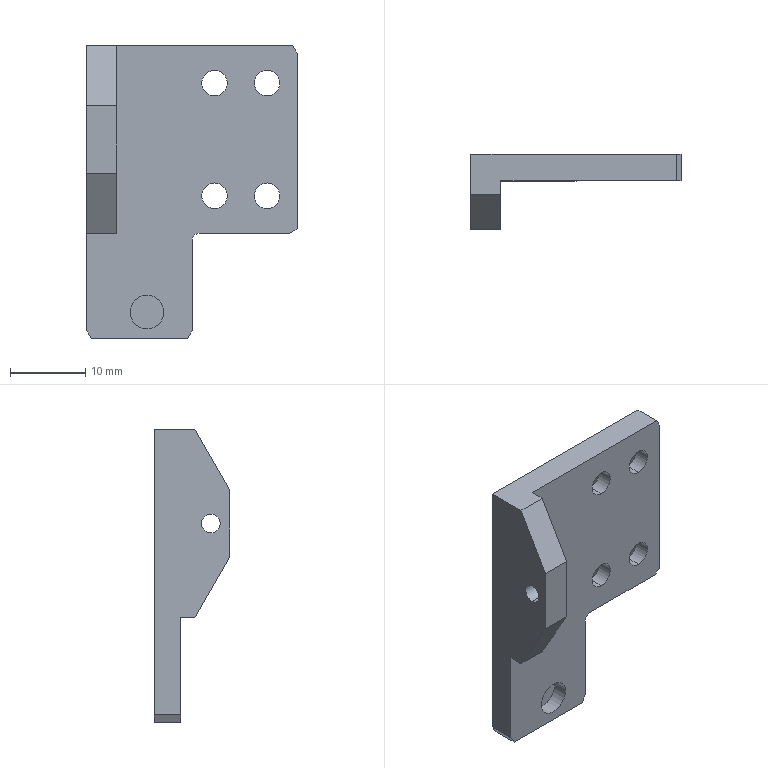Part | NX | features BREP 1 | 1 solid | 39 faces | box 28 x 10 x 39 mm | volume 3399 mm3 | plane 18 | cylinder 13 | cone 8 | commonest cylinder face diameters 3.4 x8 2.5 x2 4.5 x2 2 x1
STEP:
#1=CARTESIAN_POINT('',(15.,10.,-12.5));
#2=VERTEX_POINT('',#1);
#3=CARTESIAN_POINT('',(14.,10.,-13.5));
#4=VERTEX_POINT('',#3);
#5=CARTESIAN_POINT('',(15.,10.,-13.5));
#6=DIRECTION('',(0.,-1.,0.));
#7=DIRECTION('',(0.,0.,-1.));
#8=AXIS2_PLACEMENT_3D('',#5,#6,#7);
#9=CIRCLE('',#8,1.);
#10=EDGE_CURVE('',#2,#4,#9,.T.);
#11=ORIENTED_EDGE('',*,*,#10,.F.);
#12=CARTESIAN_POINT('',(15.,6.5,-12.5));
#13=VERTEX_POINT('',#12);
#14=CARTESIAN_POINT('',(15.,0.,-12.5));
#15=DIRECTION('',(0.,1.,0.));
#16=VECTOR('',#15,1000.);
#17=LINE('',#14,#16);
#18=EDGE_CURVE('',#13,#2,#17,.T.);
#19=ORIENTED_EDGE('',*,*,#18,.F.);
#20=CARTESIAN_POINT('',(14.,6.5,-13.5));
#21=VERTEX_POINT('',#20);
#22=CARTESIAN_POINT('',(15.,6.5,-13.5));
#23=DIRECTION('',(0.,1.,0.));
#24=DIRECTION('',(-1.,0.,0.));
#25=AXIS2_PLACEMENT_3D('',#22,#23,#24);
#26=CIRCLE('',#25,1.);
#27=EDGE_CURVE('',#21,#13,#26,.T.);
#28=ORIENTED_EDGE('',*,*,#27,.F.);
#29=CARTESIAN_POINT('',(14.,10.,-13.5));
#30=DIRECTION('',(0.,-1.,0.));
#31=VECTOR('',#30,1000.);
#32=LINE('',#29,#31);
#33=EDGE_CURVE('',#4,#21,#32,.T.);
#34=ORIENTED_EDGE('',*,*,#33,.F.);
#35=EDGE_LOOP('',(#11,#19,#28,#34));
#36=FACE_BOUND('',#35,.T.);
#37=CARTESIAN_POINT('',(15.,10.,-13.5));
#38=DIRECTION('',(0.,-1.,0.));
#39=DIRECTION('',(1.,0.,0.));
#40=AXIS2_PLACEMENT_3D('',#37,#38,#39);
#41=CYLINDRICAL_SURFACE('',#40,1.);
#42=ADVANCED_FACE('',(#36),#41,.F.);
#43=CARTESIAN_POINT('',(14.,10.,-25.5));
#44=VERTEX_POINT('',#43);
#45=CARTESIAN_POINT('',(13.423,10.,-26.5));
#46=VERTEX_POINT('',#45);
#47=CARTESIAN_POINT('',(13.423,10.,-26.5));
#48=DIRECTION('',(-0.5,0.,-0.866));
#49=VECTOR('',#48,1000.);
#50=LINE('',#47,#49);
#51=EDGE_CURVE('',#44,#46,#50,.T.);
#52=ORIENTED_EDGE('',*,*,#51,.F.);
#53=CARTESIAN_POINT('',(14.,6.5,-25.5));
#54=VERTEX_POINT('',#53);
#55=CARTESIAN_POINT('',(14.,10.,-25.5));
#56=DIRECTION('',(0.,1.,0.));
#57=VECTOR('',#56,1000.);
#58=LINE('',#55,#57);
#59=EDGE_CURVE('',#54,#44,#58,.T.);
#60=ORIENTED_EDGE('',*,*,#59,.F.);
#61=CARTESIAN_POINT('',(13.423,6.5,-26.5));
#62=VERTEX_POINT('',#61);
#63=CARTESIAN_POINT('',(13.423,6.5,-26.5));
#64=DIRECTION('',(0.5,0.,0.866));
#65=VECTOR('',#64,1000.);
#66=LINE('',#63,#65);
#67=EDGE_CURVE('',#62,#54,#66,.T.);
#68=ORIENTED_EDGE('',*,*,#67,.F.);
#69=CARTESIAN_POINT('',(13.423,0.,-26.5));
#70=DIRECTION('',(0.,-1.,0.));
#71=VECTOR('',#70,1000.);
#72=LINE('',#69,#71);
#73=EDGE_CURVE('',#46,#62,#72,.T.);
#74=ORIENTED_EDGE('',*,*,#73,.F.);
#75=EDGE_LOOP('',(#52,#60,#68,#74));
#76=FACE_BOUND('',#75,.T.);
#77=CARTESIAN_POINT('',(13.423,0.,-26.5));
#78=DIRECTION('',(-0.866,0.,0.5));
#79=DIRECTION('',(0.,-1.,0.));
#80=AXIS2_PLACEMENT_3D('',#77,#78,#79);
#81=PLANE('',#80);
#82=ADVANCED_FACE('',(#76),#81,.F.);
#83=CARTESIAN_POINT('',(0.,6.5,-25.5));
#84=VERTEX_POINT('',#83);
#85=CARTESIAN_POINT('',(0.5774,6.5,-26.5));
#86=VERTEX_POINT('',#85);
#87=CARTESIAN_POINT('',(0.5774,6.5,-26.5));
#88=DIRECTION('',(0.5,0.,-0.866));
#89=VECTOR('',#88,1000.);
#90=LINE('',#87,#89);
#91=EDGE_CURVE('',#84,#86,#90,.T.);
#92=ORIENTED_EDGE('',*,*,#91,.F.);
#93=CARTESIAN_POINT('',(0.,10.,-25.5));
#94=VERTEX_POINT('',#93);
#95=CARTESIAN_POINT('',(0.,0.,-25.5));
#96=DIRECTION('',(0.,-1.,0.));
#97=VECTOR('',#96,1000.);
#98=LINE('',#95,#97);
#99=EDGE_CURVE('',#94,#84,#98,.T.);
#100=ORIENTED_EDGE('',*,*,#99,.F.);
#101=CARTESIAN_POINT('',(0.5774,10.,-26.5));
#102=VERTEX_POINT('',#101);
#103=CARTESIAN_POINT('',(0.5774,10.,-26.5));
#104=DIRECTION('',(-0.5,0.,0.866));
#105=VECTOR('',#104,1000.);
#106=LINE('',#103,#105);
#107=EDGE_CURVE('',#102,#94,#106,.T.);
#108=ORIENTED_EDGE('',*,*,#107,.F.);
#109=CARTESIAN_POINT('',(0.5774,0.,-26.5));
#110=DIRECTION('',(0.,1.,0.));
#111=VECTOR('',#110,1000.);
#112=LINE('',#109,#111);
#113=EDGE_CURVE('',#86,#102,#112,.T.);
#114=ORIENTED_EDGE('',*,*,#113,.F.);
#115=EDGE_LOOP('',(#92,#100,#108,#114));
#116=FACE_BOUND('',#115,.T.);
#117=CARTESIAN_POINT('',(0.5774,0.,-26.5));
#118=DIRECTION('',(0.866,0.,0.5));
#119=DIRECTION('',(0.,1.,0.));
#120=AXIS2_PLACEMENT_3D('',#117,#118,#119);
#121=PLANE('',#120);
#122=ADVANCED_FACE('',(#116),#121,.F.);
#123=CARTESIAN_POINT('',(27.,6.5,-12.5));
#124=VERTEX_POINT('',#123);
#125=CARTESIAN_POINT('',(28.,6.5,-11.923));
#126=VERTEX_POINT('',#125);
#127=CARTESIAN_POINT('',(28.,6.5,-11.923));
#128=DIRECTION('',(0.866,0.,0.5));
#129=VECTOR('',#128,1000.);
#130=LINE('',#127,#129);
#131=EDGE_CURVE('',#124,#126,#130,.T.);
#132=ORIENTED_EDGE('',*,*,#131,.F.);
#133=CARTESIAN_POINT('',(27.,10.,-12.5));
#134=VERTEX_POINT('',#133);
#135=CARTESIAN_POINT('',(27.,6.5,-12.5));
#136=DIRECTION('',(0.,-1.,0.));
#137=VECTOR('',#136,1000.);
#138=LINE('',#135,#137);
#139=EDGE_CURVE('',#134,#124,#138,.T.);
#140=ORIENTED_EDGE('',*,*,#139,.F.);
#141=CARTESIAN_POINT('',(28.,10.,-11.923));
#142=VERTEX_POINT('',#141);
#143=CARTESIAN_POINT('',(28.,10.,-11.923));
#144=DIRECTION('',(-0.866,0.,-0.5));
#145=VECTOR('',#144,1000.);
#146=LINE('',#143,#145);
#147=EDGE_CURVE('',#142,#134,#146,.T.);
#148=ORIENTED_EDGE('',*,*,#147,.F.);
#149=CARTESIAN_POINT('',(28.,10.,-11.923));
#150=DIRECTION('',(0.,1.,0.));
#151=VECTOR('',#150,1000.);
#152=LINE('',#149,#151);
#153=EDGE_CURVE('',#126,#142,#152,.T.);
#154=ORIENTED_EDGE('',*,*,#153,.F.);
#155=EDGE_LOOP('',(#132,#140,#148,#154));
#156=FACE_BOUND('',#155,.T.);
#157=CARTESIAN_POINT('',(28.,10.,-11.923));
#158=DIRECTION('',(0.5,0.,-0.866));
#159=DIRECTION('',(0.,-1.,0.));
#160=AXIS2_PLACEMENT_3D('',#157,#158,#159);
#161=PLANE('',#160);
#162=ADVANCED_FACE('',(#156),#161,.T.);
#163=CARTESIAN_POINT('',(28.,6.5,11.5));
#164=VERTEX_POINT('',#163);
#165=CARTESIAN_POINT('',(27.423,6.5,12.5));
#166=VERTEX_POINT('',#165);
#167=CARTESIAN_POINT('',(27.423,6.5,12.5));
#168=DIRECTION('',(-0.5,0.,0.866));
#169=VECTOR('',#168,1000.);
#170=LINE('',#167,#169);
#171=EDGE_CURVE('',#164,#166,#170,.T.);
#172=ORIENTED_EDGE('',*,*,#171,.F.);
#173=CARTESIAN_POINT('',(28.,10.,11.5));
#174=VERTEX_POINT('',#173);
#175=CARTESIAN_POINT('',(28.,10.,11.5));
#176=DIRECTION('',(0.,-1.,0.));
#177=VECTOR('',#176,1000.);
#178=LINE('',#175,#177);
#179=EDGE_CURVE('',#174,#164,#178,.T.);
#180=ORIENTED_EDGE('',*,*,#179,.F.);
#181=CARTESIAN_POINT('',(27.423,10.,12.5));
#182=VERTEX_POINT('',#181);
#183=CARTESIAN_POINT('',(27.423,10.,12.5));
#184=DIRECTION('',(0.5,0.,-0.866));
#185=VECTOR('',#184,1000.);
#186=LINE('',#183,#185);
#187=EDGE_CURVE('',#182,#174,#186,.T.);
#188=ORIENTED_EDGE('',*,*,#187,.F.);
#189=CARTESIAN_POINT('',(27.423,0.,12.5));
#190=DIRECTION('',(0.,1.,0.));
#191=VECTOR('',#190,1000.);
#192=LINE('',#189,#191);
#193=EDGE_CURVE('',#166,#182,#192,.T.);
#194=ORIENTED_EDGE('',*,*,#193,.F.);
#195=EDGE_LOOP('',(#172,#180,#188,#194));
#196=FACE_BOUND('',#195,.T.);
#197=CARTESIAN_POINT('',(27.423,0.,12.5));
#198=DIRECTION('',(-0.866,0.,-0.5));
#199=DIRECTION('',(0.,1.,0.));
#200=AXIS2_PLACEMENT_3D('',#197,#198,#199);
#201=PLANE('',#200);
#202=ADVANCED_FACE('',(#196),#201,.F.);
#203=CARTESIAN_POINT('',(10.25,8.5,-23.));
#204=VERTEX_POINT('',#203);
#205=CARTESIAN_POINT('',(5.75,8.5,-23.));
#206=VERTEX_POINT('',#205);
#207=CARTESIAN_POINT('',(8.,8.5,-23.));
#208=DIRECTION('',(0.,-1.,0.));
#209=DIRECTION('',(1.,0.,0.));
#210=AXIS2_PLACEMENT_3D('',#207,#208,#209);
#211=CIRCLE('',#210,2.25);
#212=EDGE_CURVE('',#204,#206,#211,.T.);
#213=ORIENTED_EDGE('',*,*,#212,.T.);
#214=CARTESIAN_POINT('',(8.,8.5,-23.));
#215=DIRECTION('',(0.,-1.,0.));
#216=DIRECTION('',(1.,0.,0.));
#217=AXIS2_PLACEMENT_3D('',#214,#215,#216);
#218=CIRCLE('',#217,2.25);
#219=EDGE_CURVE('',#206,#204,#218,.T.);
#220=ORIENTED_EDGE('',*,*,#219,.T.);
#221=EDGE_LOOP('',(#213,#220));
#222=FACE_BOUND('',#221,.T.);
#223=CARTESIAN_POINT('',(8.,8.5,-23.));
#224=DIRECTION('',(0.,-1.,0.));
#225=DIRECTION('',(1.,0.,0.));
#226=AXIS2_PLACEMENT_3D('',#223,#224,#225);
#227=PLANE('',#226);
#228=ADVANCED_FACE('',(#222),#227,.T.);
#229=CARTESIAN_POINT('',(5.75,6.5,-23.));
#230=VERTEX_POINT('',#229);
#231=CARTESIAN_POINT('',(5.75,8.5,-23.));
#232=DIRECTION('',(0.,-1.,0.));
#233=VECTOR('',#232,1000.);
#234=LINE('',#231,#233);
#235=EDGE_CURVE('',#230,#206,#234,.F.);
#236=ORIENTED_EDGE('',*,*,#235,.T.);
#237=ORIENTED_EDGE('',*,*,#212,.F.);
#238=CARTESIAN_POINT('',(10.25,6.5,-23.));
#239=VERTEX_POINT('',#238);
#240=CARTESIAN_POINT('',(10.25,8.5,-23.));
#241=DIRECTION('',(0.,-1.,0.));
#242=VECTOR('',#241,1000.);
#243=LINE('',#240,#242);
#244=EDGE_CURVE('',#239,#204,#243,.F.);
#245=ORIENTED_EDGE('',*,*,#244,.F.);
#246=CARTESIAN_POINT('',(8.,6.5,-23.));
#247=DIRECTION('',(0.,-1.,0.));
#248=DIRECTION('',(1.,0.,0.));
#249=AXIS2_PLACEMENT_3D('',#246,#247,#248);
#250=CIRCLE('',#249,2.25);
#251=EDGE_CURVE('',#239,#230,#250,.T.);
#252=ORIENTED_EDGE('',*,*,#251,.T.);
#253=EDGE_LOOP('',(#236,#237,#245,#252));
#254=FACE_BOUND('',#253,.T.);
#255=CARTESIAN_POINT('',(8.,8.5,-23.));
#256=DIRECTION('',(0.,-1.,0.));
#257=DIRECTION('',(1.,0.,0.));
#258=AXIS2_PLACEMENT_3D('',#255,#256,#257);
#259=CYLINDRICAL_SURFACE('',#258,2.25);
#260=ADVANCED_FACE('',(#254),#259,.F.);
#261=CARTESIAN_POINT('',(0.,6.5,-26.5));
#262=DIRECTION('',(-1.,0.,0.));
#263=VECTOR('',#262,1000.);
#264=LINE('',#261,#263);
#265=EDGE_CURVE('',#62,#86,#264,.T.);
#266=ORIENTED_EDGE('',*,*,#265,.T.);
#267=ORIENTED_EDGE('',*,*,#113,.T.);
#268=CARTESIAN_POINT('',(0.,10.,-26.5));
#269=DIRECTION('',(1.,0.,0.));
#270=VECTOR('',#269,1000.);
#271=LINE('',#268,#270);
#272=EDGE_CURVE('',#102,#46,#271,.T.);
#273=ORIENTED_EDGE('',*,*,#272,.T.);
#274=ORIENTED_EDGE('',*,*,#73,.T.);
#275=EDGE_LOOP('',(#266,#267,#273,#274));
#276=FACE_BOUND('',#275,.T.);
#277=CARTESIAN_POINT('',(0.,0.,-26.5));
#278=DIRECTION('',(0.,0.,1.));
#279=DIRECTION('',(1.,0.,0.));
#280=AXIS2_PLACEMENT_3D('',#277,#278,#279);
#281=PLANE('',#280);
#282=ADVANCED_FACE('',(#276),#281,.F.);
#283=CARTESIAN_POINT('',(14.,10.,-26.5));
#284=DIRECTION('',(0.,0.,1.));
#285=VECTOR('',#284,1000.);
#286=LINE('',#283,#285);
#287=EDGE_CURVE('',#44,#4,#286,.T.);
#288=ORIENTED_EDGE('',*,*,#287,.T.);
#289=ORIENTED_EDGE('',*,*,#33,.T.);
#290=CARTESIAN_POINT('',(14.,6.5,-26.5));
#291=DIRECTION('',(0.,0.,1.));
#292=VECTOR('',#291,1000.);
#293=LINE('',#290,#292);
#294=EDGE_CURVE('',#54,#21,#293,.T.);
#295=ORIENTED_EDGE('',*,*,#294,.F.);
#296=ORIENTED_EDGE('',*,*,#59,.T.);
#297=EDGE_LOOP('',(#288,#289,#295,#296));
#298=FACE_BOUND('',#297,.T.);
#299=CARTESIAN_POINT('',(14.,10.,-26.5));
#300=DIRECTION('',(-1.,0.,0.));
#301=DIRECTION('',(0.,-1.,0.));
#302=AXIS2_PLACEMENT_3D('',#299,#300,#301);
#303=PLANE('',#302);
#304=ADVANCED_FACE('',(#298),#303,.F.);
#305=CARTESIAN_POINT('',(0.,0.,4.5));
#306=VERTEX_POINT('',#305);
#307=CARTESIAN_POINT('',(0.,4.619,12.5));
#308=VERTEX_POINT('',#307);
#309=CARTESIAN_POINT('',(0.,4.619,12.5));
#310=DIRECTION('',(0.,0.5,0.866));
#311=VECTOR('',#310,1000.);
#312=LINE('',#309,#311);
#313=EDGE_CURVE('',#306,#308,#312,.T.);
#314=ORIENTED_EDGE('',*,*,#313,.F.);
#315=CARTESIAN_POINT('',(4.,0.,4.5));
#316=VERTEX_POINT('',#315);
#317=CARTESIAN_POINT('',(4.,0.,4.5));
#318=DIRECTION('',(-1.,0.,0.));
#319=VECTOR('',#318,1000.);
#320=LINE('',#317,#319);
#321=EDGE_CURVE('',#316,#306,#320,.T.);
#322=ORIENTED_EDGE('',*,*,#321,.F.);
#323=CARTESIAN_POINT('',(4.,4.619,12.5));
#324=VERTEX_POINT('',#323);
#325=CARTESIAN_POINT('',(4.,4.619,12.5));
#326=DIRECTION('',(0.,-0.5,-0.866));
#327=VECTOR('',#326,1000.);
#328=LINE('',#325,#327);
#329=EDGE_CURVE('',#324,#316,#328,.T.);
#330=ORIENTED_EDGE('',*,*,#329,.F.);
#331=CARTESIAN_POINT('',(0.,4.619,12.5));
#332=DIRECTION('',(1.,0.,0.));
#333=VECTOR('',#332,1000.);
#334=LINE('',#331,#333);
#335=EDGE_CURVE('',#308,#324,#334,.T.);
#336=ORIENTED_EDGE('',*,*,#335,.F.);
#337=EDGE_LOOP('',(#314,#322,#330,#336));
#338=FACE_BOUND('',#337,.T.);
#339=CARTESIAN_POINT('',(0.,4.619,12.5));
#340=DIRECTION('',(0.,0.866,-0.5));
#341=DIRECTION('',(1.,0.,0.));
#342=AXIS2_PLACEMENT_3D('',#339,#340,#341);
#343=PLANE('',#342);
#344=ADVANCED_FACE('',(#338),#343,.F.);
#345=CARTESIAN_POINT('',(0.,4.619,-12.5));
#346=VERTEX_POINT('',#345);
#347=CARTESIAN_POINT('',(0.,0.,-4.5));
#348=VERTEX_POINT('',#347);
#349=CARTESIAN_POINT('',(0.,0.,-4.5));
#350=DIRECTION('',(0.,-0.5,0.866));
#351=VECTOR('',#350,1000.);
#352=LINE('',#349,#351);
#353=EDGE_CURVE('',#346,#348,#352,.T.);
#354=ORIENTED_EDGE('',*,*,#353,.F.);
#355=CARTESIAN_POINT('',(4.,4.619,-12.5));
#356=VERTEX_POINT('',#355);
#357=CARTESIAN_POINT('',(0.,4.619,-12.5));
#358=DIRECTION('',(-1.,0.,0.));
#359=VECTOR('',#358,1000.);
#360=LINE('',#357,#359);
#361=EDGE_CURVE('',#356,#346,#360,.T.);
#362=ORIENTED_EDGE('',*,*,#361,.F.);
#363=CARTESIAN_POINT('',(4.,0.,-4.5));
#364=VERTEX_POINT('',#363);
#365=CARTESIAN_POINT('',(4.,0.,-4.5));
#366=DIRECTION('',(0.,0.5,-0.866));
#367=VECTOR('',#366,1000.);
#368=LINE('',#365,#367);
#369=EDGE_CURVE('',#364,#356,#368,.T.);
#370=ORIENTED_EDGE('',*,*,#369,.F.);
#371=CARTESIAN_POINT('',(4.,0.,-4.5));
#372=DIRECTION('',(1.,0.,0.));
#373=VECTOR('',#372,1000.);
#374=LINE('',#371,#373);
#375=EDGE_CURVE('',#348,#364,#374,.T.);
#376=ORIENTED_EDGE('',*,*,#375,.F.);
#377=EDGE_LOOP('',(#354,#362,#370,#376));
#378=FACE_BOUND('',#377,.T.);
#379=CARTESIAN_POINT('',(4.,0.,-4.5));
#380=DIRECTION('',(0.,-0.866,-0.5));
#381=DIRECTION('',(-1.,0.,0.));
#382=AXIS2_PLACEMENT_3D('',#379,#380,#381);
#383=PLANE('',#382);
#384=ADVANCED_FACE('',(#378),#383,.T.);
#385=CARTESIAN_POINT('',(17.,10.,4.35));
#386=VERTEX_POINT('',#385);
#387=CARTESIAN_POINT('',(17.,8.55,5.8));
#388=VERTEX_POINT('',#387);
#389=CARTESIAN_POINT('',(17.,10.,4.35));
#390=DIRECTION('',(0.,0.7071,-0.7071));
#391=VECTOR('',#390,1000.);
#392=LINE('',#389,#391);
#393=EDGE_CURVE('',#386,#388,#392,.F.);
#394=ORIENTED_EDGE('',*,*,#393,.T.);
#395=CARTESIAN_POINT('',(17.,8.55,9.2));
#396=VERTEX_POINT('',#395);
#397=CARTESIAN_POINT('',(17.,8.55,7.5));
#398=DIRECTION('',(0.,1.,0.));
#399=DIRECTION('',(0.,0.,1.));
#400=AXIS2_PLACEMENT_3D('',#397,#398,#399);
#401=CIRCLE('',#400,1.7);
#402=EDGE_CURVE('',#396,#388,#401,.T.);
#403=ORIENTED_EDGE('',*,*,#402,.F.);
#404=CARTESIAN_POINT('',(17.,10.,10.65));
#405=VERTEX_POINT('',#404);
#406=CARTESIAN_POINT('',(17.,10.,10.65));
#407=DIRECTION('',(0.,0.7071,0.7071));
#408=VECTOR('',#407,1000.);
#409=LINE('',#406,#408);
#410=EDGE_CURVE('',#405,#396,#409,.F.);
#411=ORIENTED_EDGE('',*,*,#410,.F.);
#412=CARTESIAN_POINT('',(17.,10.,7.5));
#413=DIRECTION('',(0.,1.,0.));
#414=DIRECTION('',(0.,0.,1.));
#415=AXIS2_PLACEMENT_3D('',#412,#413,#414);
#416=CIRCLE('',#415,3.15);
#417=EDGE_CURVE('',#405,#386,#416,.T.);
#418=ORIENTED_EDGE('',*,*,#417,.T.);
#419=EDGE_LOOP('',(#394,#403,#411,#418));
#420=FACE_BOUND('',#419,.T.);
#421=CARTESIAN_POINT('',(17.,10.,7.5));
#422=DIRECTION('',(0.,1.,0.));
#423=DIRECTION('',(0.,0.,1.));
#424=AXIS2_PLACEMENT_3D('',#421,#422,#423);
#425=CONICAL_SURFACE('',#424,3.15,0.7854);
#426=ADVANCED_FACE('',(#420),#425,.F.);
#427=CARTESIAN_POINT('',(17.,6.5,5.8));
#428=VERTEX_POINT('',#427);
#429=CARTESIAN_POINT('',(17.,10.,5.8));
#430=DIRECTION('',(0.,1.,0.));
#431=VECTOR('',#430,1000.);
#432=LINE('',#429,#431);
#433=EDGE_CURVE('',#388,#428,#432,.F.);
#434=ORIENTED_EDGE('',*,*,#433,.T.);
#435=CARTESIAN_POINT('',(17.,6.5,9.2));
#436=VERTEX_POINT('',#435);
#437=CARTESIAN_POINT('',(17.,6.5,7.5));
#438=DIRECTION('',(0.,1.,0.));
#439=DIRECTION('',(-1.,0.,0.));
#440=AXIS2_PLACEMENT_3D('',#437,#438,#439);
#441=CIRCLE('',#440,1.7);
#442=EDGE_CURVE('',#436,#428,#441,.T.);
#443=ORIENTED_EDGE('',*,*,#442,.F.);
#444=CARTESIAN_POINT('',(17.,10.,9.2));
#445=DIRECTION('',(0.,1.,0.));
#446=VECTOR('',#445,1000.);
#447=LINE('',#444,#446);
#448=EDGE_CURVE('',#396,#436,#447,.F.);
#449=ORIENTED_EDGE('',*,*,#448,.F.);
#450=ORIENTED_EDGE('',*,*,#402,.T.);
#451=EDGE_LOOP('',(#434,#443,#449,#450));
#452=FACE_BOUND('',#451,.T.);
#453=CARTESIAN_POINT('',(17.,10.,7.5));
#454=DIRECTION('',(0.,1.,0.));
#455=DIRECTION('',(0.,0.,1.));
#456=AXIS2_PLACEMENT_3D('',#453,#454,#455);
#457=CYLINDRICAL_SURFACE('',#456,1.7);
#458=ADVANCED_FACE('',(#452),#457,.F.);
#459=CARTESIAN_POINT('',(24.,10.,4.35));
#460=VERTEX_POINT('',#459);
#461=CARTESIAN_POINT('',(24.,8.55,5.8));
#462=VERTEX_POINT('',#461);
#463=CARTESIAN_POINT('',(24.,10.,4.35));
#464=DIRECTION('',(0.,0.7071,-0.7071));
#465=VECTOR('',#464,1000.);
#466=LINE('',#463,#465);
#467=EDGE_CURVE('',#460,#462,#466,.F.);
#468=ORIENTED_EDGE('',*,*,#467,.T.);
#469=CARTESIAN_POINT('',(24.,8.55,9.2));
#470=VERTEX_POINT('',#469);
#471=CARTESIAN_POINT('',(24.,8.55,7.5));
#472=DIRECTION('',(0.,1.,0.));
#473=DIRECTION('',(0.,0.,1.));
#474=AXIS2_PLACEMENT_3D('',#471,#472,#473);
#475=CIRCLE('',#474,1.7);
#476=EDGE_CURVE('',#470,#462,#475,.T.);
#477=ORIENTED_EDGE('',*,*,#476,.F.);
#478=CARTESIAN_POINT('',(24.,10.,10.65));
#479=VERTEX_POINT('',#478);
#480=CARTESIAN_POINT('',(24.,10.,10.65));
#481=DIRECTION('',(0.,0.7071,0.7071));
#482=VECTOR('',#481,1000.);
#483=LINE('',#480,#482);
#484=EDGE_CURVE('',#479,#470,#483,.F.);
#485=ORIENTED_EDGE('',*,*,#484,.F.);
#486=CARTESIAN_POINT('',(24.,10.,7.5));
#487=DIRECTION('',(0.,1.,0.));
#488=DIRECTION('',(0.,0.,1.));
#489=AXIS2_PLACEMENT_3D('',#486,#487,#488);
#490=CIRCLE('',#489,3.15);
#491=EDGE_CURVE('',#479,#460,#490,.T.);
#492=ORIENTED_EDGE('',*,*,#491,.T.);
#493=EDGE_LOOP('',(#468,#477,#485,#492));
#494=FACE_BOUND('',#493,.T.);
#495=CARTESIAN_POINT('',(24.,10.,7.5));
#496=DIRECTION('',(0.,1.,0.));
#497=DIRECTION('',(0.,0.,1.));
#498=AXIS2_PLACEMENT_3D('',#495,#496,#497);
#499=CONICAL_SURFACE('',#498,3.15,0.7854);
#500=ADVANCED_FACE('',(#494),#499,.F.);
#501=CARTESIAN_POINT('',(24.,6.5,5.8));
#502=VERTEX_POINT('',#501);
#503=CARTESIAN_POINT('',(24.,10.,5.8));
#504=DIRECTION('',(0.,1.,0.));
#505=VECTOR('',#504,1000.);
#506=LINE('',#503,#505);
#507=EDGE_CURVE('',#462,#502,#506,.F.);
#508=ORIENTED_EDGE('',*,*,#507,.T.);
#509=CARTESIAN_POINT('',(24.,6.5,9.2));
#510=VERTEX_POINT('',#509);
#511=CARTESIAN_POINT('',(24.,6.5,7.5));
#512=DIRECTION('',(0.,1.,0.));
#513=DIRECTION('',(-1.,0.,0.));
#514=AXIS2_PLACEMENT_3D('',#511,#512,#513);
#515=CIRCLE('',#514,1.7);
#516=EDGE_CURVE('',#510,#502,#515,.T.);
#517=ORIENTED_EDGE('',*,*,#516,.F.);
#518=CARTESIAN_POINT('',(24.,10.,9.2));
#519=DIRECTION('',(0.,1.,0.));
#520=VECTOR('',#519,1000.);
#521=LINE('',#518,#520);
#522=EDGE_CURVE('',#470,#510,#521,.F.);
#523=ORIENTED_EDGE('',*,*,#522,.F.);
#524=ORIENTED_EDGE('',*,*,#476,.T.);
#525=EDGE_LOOP('',(#508,#517,#523,#524));
#526=FACE_BOUND('',#525,.T.);
#527=CARTESIAN_POINT('',(24.,10.,7.5));
#528=DIRECTION('',(0.,1.,0.));
#529=DIRECTION('',(0.,0.,1.));
#530=AXIS2_PLACEMENT_3D('',#527,#528,#529);
#531=CYLINDRICAL_SURFACE('',#530,1.7);
#532=ADVANCED_FACE('',(#526),#531,.F.);
#533=CARTESIAN_POINT('',(17.,10.,-10.65));
#534=VERTEX_POINT('',#533);
#535=CARTESIAN_POINT('',(17.,8.55,-9.2));
#536=VERTEX_POINT('',#535);
#537=CARTESIAN_POINT('',(17.,10.,-10.65));
#538=DIRECTION('',(0.,0.7071,-0.7071));
#539=VECTOR('',#538,1000.);
#540=LINE('',#537,#539);
#541=EDGE_CURVE('',#534,#536,#540,.F.);
#542=ORIENTED_EDGE('',*,*,#541,.T.);
#543=CARTESIAN_POINT('',(17.,8.55,-5.8));
#544=VERTEX_POINT('',#543);
#545=CARTESIAN_POINT('',(17.,8.55,-7.5));
#546=DIRECTION('',(0.,1.,0.));
#547=DIRECTION('',(0.,0.,1.));
#548=AXIS2_PLACEMENT_3D('',#545,#546,#547);
#549=CIRCLE('',#548,1.7);
#550=EDGE_CURVE('',#544,#536,#549,.T.);
#551=ORIENTED_EDGE('',*,*,#550,.F.);
#552=CARTESIAN_POINT('',(17.,10.,-4.35));
#553=VERTEX_POINT('',#552);
#554=CARTESIAN_POINT('',(17.,10.,-4.35));
#555=DIRECTION('',(0.,0.7071,0.7071));
#556=VECTOR('',#555,1000.);
#557=LINE('',#554,#556);
#558=EDGE_CURVE('',#553,#544,#557,.F.);
#559=ORIENTED_EDGE('',*,*,#558,.F.);
#560=CARTESIAN_POINT('',(17.,10.,-7.5));
#561=DIRECTION('',(0.,1.,0.));
#562=DIRECTION('',(0.,0.,1.));
#563=AXIS2_PLACEMENT_3D('',#560,#561,#562);
#564=CIRCLE('',#563,3.15);
#565=EDGE_CURVE('',#553,#534,#564,.T.);
#566=ORIENTED_EDGE('',*,*,#565,.T.);
#567=EDGE_LOOP('',(#542,#551,#559,#566));
#568=FACE_BOUND('',#567,.T.);
#569=CARTESIAN_POINT('',(17.,10.,-7.5));
#570=DIRECTION('',(0.,1.,0.));
#571=DIRECTION('',(0.,0.,1.));
#572=AXIS2_PLACEMENT_3D('',#569,#570,#571);
#573=CONICAL_SURFACE('',#572,3.15,0.7854);
#574=ADVANCED_FACE('',(#568),#573,.F.);
#575=CARTESIAN_POINT('',(17.,6.5,-9.2));
#576=VERTEX_POINT('',#575);
#577=CARTESIAN_POINT('',(17.,10.,-9.2));
#578=DIRECTION('',(0.,1.,0.));
#579=VECTOR('',#578,1000.);
#580=LINE('',#577,#579);
#581=EDGE_CURVE('',#536,#576,#580,.F.);
#582=ORIENTED_EDGE('',*,*,#581,.T.);
#583=CARTESIAN_POINT('',(17.,6.5,-5.8));
#584=VERTEX_POINT('',#583);
#585=CARTESIAN_POINT('',(17.,6.5,-7.5));
#586=DIRECTION('',(0.,1.,0.));
#587=DIRECTION('',(-1.,0.,0.));
#588=AXIS2_PLACEMENT_3D('',#585,#586,#587);
#589=CIRCLE('',#588,1.7);
#590=EDGE_CURVE('',#584,#576,#589,.T.);
#591=ORIENTED_EDGE('',*,*,#590,.F.);
#592=CARTESIAN_POINT('',(17.,10.,-5.8));
#593=DIRECTION('',(0.,1.,0.));
#594=VECTOR('',#593,1000.);
#595=LINE('',#592,#594);
#596=EDGE_CURVE('',#544,#584,#595,.F.);
#597=ORIENTED_EDGE('',*,*,#596,.F.);
#598=ORIENTED_EDGE('',*,*,#550,.T.);
#599=EDGE_LOOP('',(#582,#591,#597,#598));
#600=FACE_BOUND('',#599,.T.);
#601=CARTESIAN_POINT('',(17.,10.,-7.5));
#602=DIRECTION('',(0.,1.,0.));
#603=DIRECTION('',(0.,0.,1.));
#604=AXIS2_PLACEMENT_3D('',#601,#602,#603);
#605=CYLINDRICAL_SURFACE('',#604,1.7);
#606=ADVANCED_FACE('',(#600),#605,.F.);
#607=CARTESIAN_POINT('',(24.,10.,-10.65));
#608=VERTEX_POINT('',#607);
#609=CARTESIAN_POINT('',(24.,8.55,-9.2));
#610=VERTEX_POINT('',#609);
#611=CARTESIAN_POINT('',(24.,10.,-10.65));
#612=DIRECTION('',(0.,0.7071,-0.7071));
#613=VECTOR('',#612,1000.);
#614=LINE('',#611,#613);
#615=EDGE_CURVE('',#608,#610,#614,.F.);
#616=ORIENTED_EDGE('',*,*,#615,.T.);
#617=CARTESIAN_POINT('',(24.,8.55,-5.8));
#618=VERTEX_POINT('',#617);
#619=CARTESIAN_POINT('',(24.,8.55,-7.5));
#620=DIRECTION('',(0.,1.,0.));
#621=DIRECTION('',(0.,0.,1.));
#622=AXIS2_PLACEMENT_3D('',#619,#620,#621);
#623=CIRCLE('',#622,1.7);
#624=EDGE_CURVE('',#618,#610,#623,.T.);
#625=ORIENTED_EDGE('',*,*,#624,.F.);
#626=CARTESIAN_POINT('',(24.,10.,-4.35));
#627=VERTEX_POINT('',#626);
#628=CARTESIAN_POINT('',(24.,10.,-4.35));
#629=DIRECTION('',(0.,0.7071,0.7071));
#630=VECTOR('',#629,1000.);
#631=LINE('',#628,#630);
#632=EDGE_CURVE('',#627,#618,#631,.F.);
#633=ORIENTED_EDGE('',*,*,#632,.F.);
#634=CARTESIAN_POINT('',(24.,10.,-7.5));
#635=DIRECTION('',(0.,1.,0.));
#636=DIRECTION('',(0.,0.,1.));
#637=AXIS2_PLACEMENT_3D('',#634,#635,#636);
#638=CIRCLE('',#637,3.15);
#639=EDGE_CURVE('',#627,#608,#638,.T.);
#640=ORIENTED_EDGE('',*,*,#639,.T.);
#641=EDGE_LOOP('',(#616,#625,#633,#640));
#642=FACE_BOUND('',#641,.T.);
#643=CARTESIAN_POINT('',(24.,10.,-7.5));
#644=DIRECTION('',(0.,1.,0.));
#645=DIRECTION('',(0.,0.,1.));
#646=AXIS2_PLACEMENT_3D('',#643,#644,#645);
#647=CONICAL_SURFACE('',#646,3.15,0.7854);
#648=ADVANCED_FACE('',(#642),#647,.F.);
#649=CARTESIAN_POINT('',(24.,6.5,-9.2));
#650=VERTEX_POINT('',#649);
#651=CARTESIAN_POINT('',(24.,10.,-9.2));
#652=DIRECTION('',(0.,1.,0.));
#653=VECTOR('',#652,1000.);
#654=LINE('',#651,#653);
#655=EDGE_CURVE('',#610,#650,#654,.F.);
#656=ORIENTED_EDGE('',*,*,#655,.T.);
#657=CARTESIAN_POINT('',(24.,6.5,-5.8));
#658=VERTEX_POINT('',#657);
#659=CARTESIAN_POINT('',(24.,6.5,-7.5));
#660=DIRECTION('',(0.,1.,0.));
#661=DIRECTION('',(-1.,0.,0.));
#662=AXIS2_PLACEMENT_3D('',#659,#660,#661);
#663=CIRCLE('',#662,1.7);
#664=EDGE_CURVE('',#658,#650,#663,.T.);
#665=ORIENTED_EDGE('',*,*,#664,.F.);
#666=CARTESIAN_POINT('',(24.,10.,-5.8));
#667=DIRECTION('',(0.,1.,0.));
#668=VECTOR('',#667,1000.);
#669=LINE('',#666,#668);
#670=EDGE_CURVE('',#618,#658,#669,.F.);
#671=ORIENTED_EDGE('',*,*,#670,.F.);
#672=ORIENTED_EDGE('',*,*,#624,.T.);
#673=EDGE_LOOP('',(#656,#665,#671,#672));
#674=FACE_BOUND('',#673,.T.);
#675=CARTESIAN_POINT('',(24.,10.,-7.5));
#676=DIRECTION('',(0.,1.,0.));
#677=DIRECTION('',(0.,0.,1.));
#678=AXIS2_PLACEMENT_3D('',#675,#676,#677);
#679=CYLINDRICAL_SURFACE('',#678,1.7);
#680=ADVANCED_FACE('',(#674),#679,.F.);
#681=CARTESIAN_POINT('',(0.,2.5,-1.25));
#682=VERTEX_POINT('',#681);
#683=CARTESIAN_POINT('',(4.,2.5,-1.25));
#684=VERTEX_POINT('',#683);
#685=CARTESIAN_POINT('',(0.,2.5,-1.25));
#686=DIRECTION('',(-1.,0.,0.));
#687=VECTOR('',#686,1000.);
#688=LINE('',#685,#687);
#689=EDGE_CURVE('',#682,#684,#688,.F.);
#690=ORIENTED_EDGE('',*,*,#689,.T.);
#691=CARTESIAN_POINT('',(4.,2.5,1.25));
#692=VERTEX_POINT('',#691);
#693=CARTESIAN_POINT('',(4.,2.5,0.));
#694=DIRECTION('',(-1.,0.,0.));
#695=DIRECTION('',(0.,0.,1.));
#696=AXIS2_PLACEMENT_3D('',#693,#694,#695);
#697=CIRCLE('',#696,1.25);
#698=EDGE_CURVE('',#692,#684,#697,.T.);
#699=ORIENTED_EDGE('',*,*,#698,.F.);
#700=CARTESIAN_POINT('',(0.,2.5,1.25));
#701=VERTEX_POINT('',#700);
#702=CARTESIAN_POINT('',(0.,2.5,1.25));
#703=DIRECTION('',(-1.,0.,0.));
#704=VECTOR('',#703,1000.);
#705=LINE('',#702,#704);
#706=EDGE_CURVE('',#701,#692,#705,.F.);
#707=ORIENTED_EDGE('',*,*,#706,.F.);
#708=CARTESIAN_POINT('',(0.,2.5,0.));
#709=DIRECTION('',(-1.,0.,0.));
#710=DIRECTION('',(0.,0.,1.));
#711=AXIS2_PLACEMENT_3D('',#708,#709,#710);
#712=CIRCLE('',#711,1.25);
#713=EDGE_CURVE('',#701,#682,#712,.T.);
#714=ORIENTED_EDGE('',*,*,#713,.T.);
#715=EDGE_LOOP('',(#690,#699,#707,#714));
#716=FACE_BOUND('',#715,.T.);
#717=CARTESIAN_POINT('',(0.,2.5,0.));
#718=DIRECTION('',(-1.,0.,0.));
#719=DIRECTION('',(0.,0.,1.));
#720=AXIS2_PLACEMENT_3D('',#717,#718,#719);
#721=CYLINDRICAL_SURFACE('',#720,1.25);
#722=ADVANCED_FACE('',(#716),#721,.F.);
#723=CARTESIAN_POINT('',(28.,6.5,-12.5));
#724=DIRECTION('',(1.,0.,0.));
#725=VECTOR('',#724,1000.);
#726=LINE('',#723,#725);
#727=EDGE_CURVE('',#13,#124,#726,.T.);
#728=ORIENTED_EDGE('',*,*,#727,.F.);
#729=ORIENTED_EDGE('',*,*,#18,.T.);
#730=CARTESIAN_POINT('',(0.,10.,-12.5));
#731=DIRECTION('',(-1.,0.,0.));
#732=VECTOR('',#731,1000.);
#733=LINE('',#730,#732);
#734=EDGE_CURVE('',#134,#2,#733,.T.);
#735=ORIENTED_EDGE('',*,*,#734,.F.);
#736=ORIENTED_EDGE('',*,*,#139,.T.);
#737=EDGE_LOOP('',(#728,#729,#735,#736));
#738=FACE_BOUND('',#737,.T.);
#739=CARTESIAN_POINT('',(0.,0.,-12.5));
#740=DIRECTION('',(0.,0.,-1.));
#741=DIRECTION('',(-1.,0.,0.));
#742=AXIS2_PLACEMENT_3D('',#739,#740,#741);
#743=PLANE('',#742);
#744=ADVANCED_FACE('',(#738),#743,.T.);
#745=CARTESIAN_POINT('',(4.,6.5,12.5));
#746=VERTEX_POINT('',#745);
#747=CARTESIAN_POINT('',(28.,6.5,12.5));
#748=DIRECTION('',(1.,0.,0.));
#749=VECTOR('',#748,1000.);
#750=LINE('',#747,#749);
#751=EDGE_CURVE('',#746,#166,#750,.T.);
#752=ORIENTED_EDGE('',*,*,#751,.T.);
#753=ORIENTED_EDGE('',*,*,#193,.T.);
#754=CARTESIAN_POINT('',(0.,10.,12.5));
#755=VERTEX_POINT('',#754);
#756=CARTESIAN_POINT('',(0.,10.,12.5));
#757=DIRECTION('',(-1.,0.,0.));
#758=VECTOR('',#757,1000.);
#759=LINE('',#756,#758);
#760=EDGE_CURVE('',#182,#755,#759,.T.);
#761=ORIENTED_EDGE('',*,*,#760,.T.);
#762=CARTESIAN_POINT('',(0.,0.,12.5));
#763=DIRECTION('',(0.,-1.,0.));
#764=VECTOR('',#763,1000.);
#765=LINE('',#762,#764);
#766=EDGE_CURVE('',#755,#308,#765,.T.);
#767=ORIENTED_EDGE('',*,*,#766,.T.);
#768=ORIENTED_EDGE('',*,*,#335,.T.);
#769=CARTESIAN_POINT('',(4.,6.5,12.5));
#770=DIRECTION('',(0.,1.,0.));
#771=VECTOR('',#770,1000.);
#772=LINE('',#769,#771);
#773=EDGE_CURVE('',#324,#746,#772,.T.);
#774=ORIENTED_EDGE('',*,*,#773,.T.);
#775=EDGE_LOOP('',(#752,#753,#761,#767,#768,#774));
#776=FACE_BOUND('',#775,.T.);
#777=CARTESIAN_POINT('',(0.,0.,12.5));
#778=DIRECTION('',(0.,0.,-1.));
#779=DIRECTION('',(-1.,0.,0.));
#780=AXIS2_PLACEMENT_3D('',#777,#778,#779);
#781=PLANE('',#780);
#782=ADVANCED_FACE('',(#776),#781,.F.);
#783=CARTESIAN_POINT('',(0.,10.,12.5));
#784=DIRECTION('',(0.,0.,-1.));
#785=VECTOR('',#784,1000.);
#786=LINE('',#783,#785);
#787=EDGE_CURVE('',#755,#94,#786,.T.);
#788=ORIENTED_EDGE('',*,*,#787,.T.);
#789=ORIENTED_EDGE('',*,*,#99,.T.);
#790=CARTESIAN_POINT('',(0.,6.5,-12.5));
#791=VERTEX_POINT('',#790);
#792=CARTESIAN_POINT('',(0.,6.5,-26.5));
#793=DIRECTION('',(0.,0.,1.));
#794=VECTOR('',#793,1000.);
#795=LINE('',#792,#794);
#796=EDGE_CURVE('',#84,#791,#795,.T.);
#797=ORIENTED_EDGE('',*,*,#796,.T.);
#798=CARTESIAN_POINT('',(0.,0.,-12.5));
#799=DIRECTION('',(0.,-1.,0.));
#800=VECTOR('',#799,1000.);
#801=LINE('',#798,#800);
#802=EDGE_CURVE('',#791,#346,#801,.T.);
#803=ORIENTED_EDGE('',*,*,#802,.T.);
#804=ORIENTED_EDGE('',*,*,#353,.T.);
#805=CARTESIAN_POINT('',(0.,0.,12.5));
#806=DIRECTION('',(0.,0.,-1.));
#807=VECTOR('',#806,1000.);
#808=LINE('',#805,#807);
#809=EDGE_CURVE('',#306,#348,#808,.T.);
#810=ORIENTED_EDGE('',*,*,#809,.F.);
#811=ORIENTED_EDGE('',*,*,#313,.T.);
#812=ORIENTED_EDGE('',*,*,#766,.F.);
#813=EDGE_LOOP('',(#788,#789,#797,#803,#804,#810,#811,#812));
#814=FACE_BOUND('',#813,.T.);
#815=ORIENTED_EDGE('',*,*,#713,.F.);
#816=CARTESIAN_POINT('',(0.,2.5,0.));
#817=DIRECTION('',(-1.,0.,0.));
#818=DIRECTION('',(0.,0.,1.));
#819=AXIS2_PLACEMENT_3D('',#816,#817,#818);
#820=CIRCLE('',#819,1.25);
#821=EDGE_CURVE('',#682,#701,#820,.T.);
#822=ORIENTED_EDGE('',*,*,#821,.F.);
#823=EDGE_LOOP('',(#815,#822));
#824=FACE_BOUND('',#823,.T.);
#825=CARTESIAN_POINT('',(0.,0.,12.5));
#826=DIRECTION('',(1.,0.,0.));
#827=DIRECTION('',(0.,0.,-1.));
#828=AXIS2_PLACEMENT_3D('',#825,#826,#827);
#829=PLANE('',#828);
#830=ADVANCED_FACE('',(#814,#824),#829,.F.);
#831=ORIENTED_EDGE('',*,*,#760,.F.);
#832=ORIENTED_EDGE('',*,*,#187,.T.);
#833=CARTESIAN_POINT('',(28.,10.,12.5));
#834=DIRECTION('',(0.,0.,-1.));
#835=VECTOR('',#834,1000.);
#836=LINE('',#833,#835);
#837=EDGE_CURVE('',#174,#142,#836,.T.);
#838=ORIENTED_EDGE('',*,*,#837,.T.);
#839=ORIENTED_EDGE('',*,*,#147,.T.);
#840=ORIENTED_EDGE('',*,*,#734,.T.);
#841=ORIENTED_EDGE('',*,*,#10,.T.);
#842=ORIENTED_EDGE('',*,*,#287,.F.);
#843=ORIENTED_EDGE('',*,*,#51,.T.);
#844=ORIENTED_EDGE('',*,*,#272,.F.);
#845=ORIENTED_EDGE('',*,*,#107,.T.);
#846=ORIENTED_EDGE('',*,*,#787,.F.);
#847=EDGE_LOOP('',(#831,#832,#838,#839,#840,#841,#842,#843,#844,#845,#846));
#848=FACE_BOUND('',#847,.T.);
#849=ORIENTED_EDGE('',*,*,#639,.F.);
#850=CARTESIAN_POINT('',(24.,10.,-7.5));
#851=DIRECTION('',(0.,1.,0.));
#852=DIRECTION('',(0.,0.,1.));
#853=AXIS2_PLACEMENT_3D('',#850,#851,#852);
#854=CIRCLE('',#853,3.15);
#855=EDGE_CURVE('',#608,#627,#854,.T.);
#856=ORIENTED_EDGE('',*,*,#855,.F.);
#857=EDGE_LOOP('',(#849,#856));
#858=FACE_BOUND('',#857,.T.);
#859=ORIENTED_EDGE('',*,*,#565,.F.);
#860=CARTESIAN_POINT('',(17.,10.,-7.5));
#861=DIRECTION('',(0.,1.,0.));
#862=DIRECTION('',(0.,0.,1.));
#863=AXIS2_PLACEMENT_3D('',#860,#861,#862);
#864=CIRCLE('',#863,3.15);
#865=EDGE_CURVE('',#534,#553,#864,.T.);
#866=ORIENTED_EDGE('',*,*,#865,.F.);
#867=EDGE_LOOP('',(#859,#866));
#868=FACE_BOUND('',#867,.T.);
#869=ORIENTED_EDGE('',*,*,#491,.F.);
#870=CARTESIAN_POINT('',(24.,10.,7.5));
#871=DIRECTION('',(0.,1.,0.));
#872=DIRECTION('',(0.,0.,1.));
#873=AXIS2_PLACEMENT_3D('',#870,#871,#872);
#874=CIRCLE('',#873,3.15);
#875=EDGE_CURVE('',#460,#479,#874,.T.);
#876=ORIENTED_EDGE('',*,*,#875,.F.);
#877=EDGE_LOOP('',(#869,#876));
#878=FACE_BOUND('',#877,.T.);
#879=ORIENTED_EDGE('',*,*,#417,.F.);
#880=CARTESIAN_POINT('',(17.,10.,7.5));
#881=DIRECTION('',(0.,1.,0.));
#882=DIRECTION('',(0.,0.,1.));
#883=AXIS2_PLACEMENT_3D('',#880,#881,#882);
#884=CIRCLE('',#883,3.15);
#885=EDGE_CURVE('',#386,#405,#884,.T.);
#886=ORIENTED_EDGE('',*,*,#885,.F.);
#887=EDGE_LOOP('',(#879,#886));
#888=FACE_BOUND('',#887,.T.);
#889=CARTESIAN_POINT('',(0.,10.,12.5));
#890=DIRECTION('',(0.,-1.,0.));
#891=DIRECTION('',(0.,0.,-1.));
#892=AXIS2_PLACEMENT_3D('',#889,#890,#891);
#893=PLANE('',#892);
#894=ADVANCED_FACE('',(#848,#858,#868,#878,#888),#893,.F.);
#895=ORIENTED_EDGE('',*,*,#837,.F.);
#896=ORIENTED_EDGE('',*,*,#179,.T.);
#897=CARTESIAN_POINT('',(28.,6.5,12.5));
#898=DIRECTION('',(0.,0.,-1.));
#899=VECTOR('',#898,1000.);
#900=LINE('',#897,#899);
#901=EDGE_CURVE('',#164,#126,#900,.T.);
#902=ORIENTED_EDGE('',*,*,#901,.T.);
#903=ORIENTED_EDGE('',*,*,#153,.T.);
#904=EDGE_LOOP('',(#895,#896,#902,#903));
#905=FACE_BOUND('',#904,.T.);
#906=CARTESIAN_POINT('',(28.,10.,12.5));
#907=DIRECTION('',(-1.,0.,0.));
#908=DIRECTION('',(0.,-1.,0.));
#909=AXIS2_PLACEMENT_3D('',#906,#907,#908);
#910=PLANE('',#909);
#911=ADVANCED_FACE('',(#905),#910,.F.);
#912=ORIENTED_EDGE('',*,*,#901,.F.);
#913=ORIENTED_EDGE('',*,*,#171,.T.);
#914=ORIENTED_EDGE('',*,*,#751,.F.);
#915=CARTESIAN_POINT('',(4.,6.5,-12.5));
#916=VERTEX_POINT('',#915);
#917=CARTESIAN_POINT('',(4.,6.5,12.5));
#918=DIRECTION('',(0.,0.,-1.));
#919=VECTOR('',#918,1000.);
#920=LINE('',#917,#919);
#921=EDGE_CURVE('',#746,#916,#920,.T.);
#922=ORIENTED_EDGE('',*,*,#921,.T.);
#923=CARTESIAN_POINT('',(0.,6.5,-12.5));
#924=DIRECTION('',(-1.,0.,0.));
#925=VECTOR('',#924,1000.);
#926=LINE('',#923,#925);
#927=EDGE_CURVE('',#916,#791,#926,.T.);
#928=ORIENTED_EDGE('',*,*,#927,.T.);
#929=ORIENTED_EDGE('',*,*,#796,.F.);
#930=ORIENTED_EDGE('',*,*,#91,.T.);
#931=ORIENTED_EDGE('',*,*,#265,.F.);
#932=ORIENTED_EDGE('',*,*,#67,.T.);
#933=ORIENTED_EDGE('',*,*,#294,.T.);
#934=ORIENTED_EDGE('',*,*,#27,.T.);
#935=ORIENTED_EDGE('',*,*,#727,.T.);
#936=ORIENTED_EDGE('',*,*,#131,.T.);
#937=EDGE_LOOP('',(#912,#913,#914,#922,#928,#929,#930,#931,#932,#933,#934,#935,#936));
#938=FACE_BOUND('',#937,.T.);
#939=ORIENTED_EDGE('',*,*,#664,.T.);
#940=CARTESIAN_POINT('',(24.,6.5,-7.5));
#941=DIRECTION('',(0.,1.,0.));
#942=DIRECTION('',(-1.,0.,0.));
#943=AXIS2_PLACEMENT_3D('',#940,#941,#942);
#944=CIRCLE('',#943,1.7);
#945=EDGE_CURVE('',#650,#658,#944,.T.);
#946=ORIENTED_EDGE('',*,*,#945,.T.);
#947=EDGE_LOOP('',(#939,#946));
#948=FACE_BOUND('',#947,.T.);
#949=ORIENTED_EDGE('',*,*,#590,.T.);
#950=CARTESIAN_POINT('',(17.,6.5,-7.5));
#951=DIRECTION('',(0.,1.,0.));
#952=DIRECTION('',(-1.,0.,0.));
#953=AXIS2_PLACEMENT_3D('',#950,#951,#952);
#954=CIRCLE('',#953,1.7);
#955=EDGE_CURVE('',#576,#584,#954,.T.);
#956=ORIENTED_EDGE('',*,*,#955,.T.);
#957=EDGE_LOOP('',(#949,#956));
#958=FACE_BOUND('',#957,.T.);
#959=ORIENTED_EDGE('',*,*,#516,.T.);
#960=CARTESIAN_POINT('',(24.,6.5,7.5));
#961=DIRECTION('',(0.,1.,0.));
#962=DIRECTION('',(-1.,0.,0.));
#963=AXIS2_PLACEMENT_3D('',#960,#961,#962);
#964=CIRCLE('',#963,1.7);
#965=EDGE_CURVE('',#502,#510,#964,.T.);
#966=ORIENTED_EDGE('',*,*,#965,.T.);
#967=EDGE_LOOP('',(#959,#966));
#968=FACE_BOUND('',#967,.T.);
#969=ORIENTED_EDGE('',*,*,#442,.T.);
#970=CARTESIAN_POINT('',(17.,6.5,7.5));
#971=DIRECTION('',(0.,1.,0.));
#972=DIRECTION('',(-1.,0.,0.));
#973=AXIS2_PLACEMENT_3D('',#970,#971,#972);
#974=CIRCLE('',#973,1.7);
#975=EDGE_CURVE('',#428,#436,#974,.T.);
#976=ORIENTED_EDGE('',*,*,#975,.T.);
#977=EDGE_LOOP('',(#969,#976));
#978=FACE_BOUND('',#977,.T.);
#979=ORIENTED_EDGE('',*,*,#251,.F.);
#980=CARTESIAN_POINT('',(8.,6.5,-23.));
#981=DIRECTION('',(0.,-1.,0.));
#982=DIRECTION('',(1.,0.,0.));
#983=AXIS2_PLACEMENT_3D('',#980,#981,#982);
#984=CIRCLE('',#983,2.25);
#985=EDGE_CURVE('',#230,#239,#984,.T.);
#986=ORIENTED_EDGE('',*,*,#985,.F.);
#987=EDGE_LOOP('',(#979,#986));
#988=FACE_BOUND('',#987,.T.);
#989=CARTESIAN_POINT('',(28.,6.5,12.5));
#990=DIRECTION('',(0.,1.,0.));
#991=DIRECTION('',(-1.,0.,0.));
#992=AXIS2_PLACEMENT_3D('',#989,#990,#991);
#993=PLANE('',#992);
#994=ADVANCED_FACE('',(#938,#948,#958,#968,#978,#988),#993,.F.);
#995=CARTESIAN_POINT('',(4.,0.,12.5));
#996=DIRECTION('',(0.,0.,-1.));
#997=VECTOR('',#996,1000.);
#998=LINE('',#995,#997);
#999=EDGE_CURVE('',#316,#364,#998,.T.);
#1000=ORIENTED_EDGE('',*,*,#999,.T.);
#1001=ORIENTED_EDGE('',*,*,#369,.T.);
#1002=CARTESIAN_POINT('',(4.,6.5,-12.5));
#1003=DIRECTION('',(0.,1.,0.));
#1004=VECTOR('',#1003,1000.);
#1005=LINE('',#1002,#1004);
#1006=EDGE_CURVE('',#356,#916,#1005,.T.);
#1007=ORIENTED_EDGE('',*,*,#1006,.T.);
#1008=ORIENTED_EDGE('',*,*,#921,.F.);
#1009=ORIENTED_EDGE('',*,*,#773,.F.);
#1010=ORIENTED_EDGE('',*,*,#329,.T.);
#1011=EDGE_LOOP('',(#1000,#1001,#1007,#1008,#1009,#1010));
#1012=FACE_BOUND('',#1011,.T.);
#1013=ORIENTED_EDGE('',*,*,#698,.T.);
#1014=CARTESIAN_POINT('',(4.,2.5,0.));
#1015=DIRECTION('',(-1.,0.,0.));
#1016=DIRECTION('',(0.,0.,1.));
#1017=AXIS2_PLACEMENT_3D('',#1014,#1015,#1016);
#1018=CIRCLE('',#1017,1.25);
#1019=EDGE_CURVE('',#684,#692,#1018,.T.);
#1020=ORIENTED_EDGE('',*,*,#1019,.T.);
#1021=EDGE_LOOP('',(#1013,#1020));
#1022=FACE_BOUND('',#1021,.T.);
#1023=CARTESIAN_POINT('',(4.,6.5,12.5));
#1024=DIRECTION('',(-1.,0.,0.));
#1025=DIRECTION('',(0.,0.,1.));
#1026=AXIS2_PLACEMENT_3D('',#1023,#1024,#1025);
#1027=PLANE('',#1026);
#1028=ADVANCED_FACE('',(#1012,#1022),#1027,.F.);
#1029=ORIENTED_EDGE('',*,*,#809,.T.);
#1030=ORIENTED_EDGE('',*,*,#375,.T.);
#1031=ORIENTED_EDGE('',*,*,#999,.F.);
#1032=ORIENTED_EDGE('',*,*,#321,.T.);
#1033=EDGE_LOOP('',(#1029,#1030,#1031,#1032));
#1034=FACE_BOUND('',#1033,.T.);
#1035=CARTESIAN_POINT('',(4.,0.,12.5));
#1036=DIRECTION('',(0.,1.,0.));
#1037=DIRECTION('',(0.,0.,1.));
#1038=AXIS2_PLACEMENT_3D('',#1035,#1036,#1037);
#1039=PLANE('',#1038);
#1040=ADVANCED_FACE('',(#1034),#1039,.F.);
#1041=ORIENTED_EDGE('',*,*,#927,.F.);
#1042=ORIENTED_EDGE('',*,*,#1006,.F.);
#1043=ORIENTED_EDGE('',*,*,#361,.T.);
#1044=ORIENTED_EDGE('',*,*,#802,.F.);
#1045=EDGE_LOOP('',(#1041,#1042,#1043,#1044));
#1046=FACE_BOUND('',#1045,.T.);
#1047=CARTESIAN_POINT('',(0.,0.,-12.5));
#1048=DIRECTION('',(0.,0.,-1.));
#1049=DIRECTION('',(-1.,0.,0.));
#1050=AXIS2_PLACEMENT_3D('',#1047,#1048,#1049);
#1051=PLANE('',#1050);
#1052=ADVANCED_FACE('',(#1046),#1051,.T.);
#1053=ORIENTED_EDGE('',*,*,#1019,.F.);
#1054=ORIENTED_EDGE('',*,*,#689,.F.);
#1055=ORIENTED_EDGE('',*,*,#821,.T.);
#1056=ORIENTED_EDGE('',*,*,#706,.T.);
#1057=EDGE_LOOP('',(#1053,#1054,#1055,#1056));
#1058=FACE_BOUND('',#1057,.T.);
#1059=CARTESIAN_POINT('',(0.,2.5,0.));
#1060=DIRECTION('',(-1.,0.,0.));
#1061=DIRECTION('',(0.,0.,1.));
#1062=AXIS2_PLACEMENT_3D('',#1059,#1060,#1061);
#1063=CYLINDRICAL_SURFACE('',#1062,1.25);
#1064=ADVANCED_FACE('',(#1058),#1063,.F.);
#1065=ORIENTED_EDGE('',*,*,#945,.F.);
#1066=ORIENTED_EDGE('',*,*,#655,.F.);
#1067=CARTESIAN_POINT('',(24.,8.55,-7.5));
#1068=DIRECTION('',(0.,1.,0.));
#1069=DIRECTION('',(0.,0.,1.));
#1070=AXIS2_PLACEMENT_3D('',#1067,#1068,#1069);
#1071=CIRCLE('',#1070,1.7);
#1072=EDGE_CURVE('',#610,#618,#1071,.T.);
#1073=ORIENTED_EDGE('',*,*,#1072,.T.);
#1074=ORIENTED_EDGE('',*,*,#670,.T.);
#1075=EDGE_LOOP('',(#1065,#1066,#1073,#1074));
#1076=FACE_BOUND('',#1075,.T.);
#1077=CARTESIAN_POINT('',(24.,10.,-7.5));
#1078=DIRECTION('',(0.,1.,0.));
#1079=DIRECTION('',(0.,0.,1.));
#1080=AXIS2_PLACEMENT_3D('',#1077,#1078,#1079);
#1081=CYLINDRICAL_SURFACE('',#1080,1.7);
#1082=ADVANCED_FACE('',(#1076),#1081,.F.);
#1083=ORIENTED_EDGE('',*,*,#1072,.F.);
#1084=ORIENTED_EDGE('',*,*,#615,.F.);
#1085=ORIENTED_EDGE('',*,*,#855,.T.);
#1086=ORIENTED_EDGE('',*,*,#632,.T.);
#1087=EDGE_LOOP('',(#1083,#1084,#1085,#1086));
#1088=FACE_BOUND('',#1087,.T.);
#1089=CARTESIAN_POINT('',(24.,10.,-7.5));
#1090=DIRECTION('',(0.,1.,0.));
#1091=DIRECTION('',(0.,0.,1.));
#1092=AXIS2_PLACEMENT_3D('',#1089,#1090,#1091);
#1093=CONICAL_SURFACE('',#1092,3.15,0.7854);
#1094=ADVANCED_FACE('',(#1088),#1093,.F.);
#1095=ORIENTED_EDGE('',*,*,#955,.F.);
#1096=ORIENTED_EDGE('',*,*,#581,.F.);
#1097=CARTESIAN_POINT('',(17.,8.55,-7.5));
#1098=DIRECTION('',(0.,1.,0.));
#1099=DIRECTION('',(0.,0.,1.));
#1100=AXIS2_PLACEMENT_3D('',#1097,#1098,#1099);
#1101=CIRCLE('',#1100,1.7);
#1102=EDGE_CURVE('',#536,#544,#1101,.T.);
#1103=ORIENTED_EDGE('',*,*,#1102,.T.);
#1104=ORIENTED_EDGE('',*,*,#596,.T.);
#1105=EDGE_LOOP('',(#1095,#1096,#1103,#1104));
#1106=FACE_BOUND('',#1105,.T.);
#1107=CARTESIAN_POINT('',(17.,10.,-7.5));
#1108=DIRECTION('',(0.,1.,0.));
#1109=DIRECTION('',(0.,0.,1.));
#1110=AXIS2_PLACEMENT_3D('',#1107,#1108,#1109);
#1111=CYLINDRICAL_SURFACE('',#1110,1.7);
#1112=ADVANCED_FACE('',(#1106),#1111,.F.);
#1113=ORIENTED_EDGE('',*,*,#1102,.F.);
#1114=ORIENTED_EDGE('',*,*,#541,.F.);
#1115=ORIENTED_EDGE('',*,*,#865,.T.);
#1116=ORIENTED_EDGE('',*,*,#558,.T.);
#1117=EDGE_LOOP('',(#1113,#1114,#1115,#1116));
#1118=FACE_BOUND('',#1117,.T.);
#1119=CARTESIAN_POINT('',(17.,10.,-7.5));
#1120=DIRECTION('',(0.,1.,0.));
#1121=DIRECTION('',(0.,0.,1.));
#1122=AXIS2_PLACEMENT_3D('',#1119,#1120,#1121);
#1123=CONICAL_SURFACE('',#1122,3.15,0.7854);
#1124=ADVANCED_FACE('',(#1118),#1123,.F.);
#1125=ORIENTED_EDGE('',*,*,#965,.F.);
#1126=ORIENTED_EDGE('',*,*,#507,.F.);
#1127=CARTESIAN_POINT('',(24.,8.55,7.5));
#1128=DIRECTION('',(0.,1.,0.));
#1129=DIRECTION('',(0.,0.,1.));
#1130=AXIS2_PLACEMENT_3D('',#1127,#1128,#1129);
#1131=CIRCLE('',#1130,1.7);
#1132=EDGE_CURVE('',#462,#470,#1131,.T.);
#1133=ORIENTED_EDGE('',*,*,#1132,.T.);
#1134=ORIENTED_EDGE('',*,*,#522,.T.);
#1135=EDGE_LOOP('',(#1125,#1126,#1133,#1134));
#1136=FACE_BOUND('',#1135,.T.);
#1137=CARTESIAN_POINT('',(24.,10.,7.5));
#1138=DIRECTION('',(0.,1.,0.));
#1139=DIRECTION('',(0.,0.,1.));
#1140=AXIS2_PLACEMENT_3D('',#1137,#1138,#1139);
#1141=CYLINDRICAL_SURFACE('',#1140,1.7);
#1142=ADVANCED_FACE('',(#1136),#1141,.F.);
#1143=ORIENTED_EDGE('',*,*,#1132,.F.);
#1144=ORIENTED_EDGE('',*,*,#467,.F.);
#1145=ORIENTED_EDGE('',*,*,#875,.T.);
#1146=ORIENTED_EDGE('',*,*,#484,.T.);
#1147=EDGE_LOOP('',(#1143,#1144,#1145,#1146));
#1148=FACE_BOUND('',#1147,.T.);
#1149=CARTESIAN_POINT('',(24.,10.,7.5));
#1150=DIRECTION('',(0.,1.,0.));
#1151=DIRECTION('',(0.,0.,1.));
#1152=AXIS2_PLACEMENT_3D('',#1149,#1150,#1151);
#1153=CONICAL_SURFACE('',#1152,3.15,0.7854);
#1154=ADVANCED_FACE('',(#1148),#1153,.F.);
#1155=ORIENTED_EDGE('',*,*,#975,.F.);
#1156=ORIENTED_EDGE('',*,*,#433,.F.);
#1157=CARTESIAN_POINT('',(17.,8.55,7.5));
#1158=DIRECTION('',(0.,1.,0.));
#1159=DIRECTION('',(0.,0.,1.));
#1160=AXIS2_PLACEMENT_3D('',#1157,#1158,#1159);
#1161=CIRCLE('',#1160,1.7);
#1162=EDGE_CURVE('',#388,#396,#1161,.T.);
#1163=ORIENTED_EDGE('',*,*,#1162,.T.);
#1164=ORIENTED_EDGE('',*,*,#448,.T.);
#1165=EDGE_LOOP('',(#1155,#1156,#1163,#1164));
#1166=FACE_BOUND('',#1165,.T.);
#1167=CARTESIAN_POINT('',(17.,10.,7.5));
#1168=DIRECTION('',(0.,1.,0.));
#1169=DIRECTION('',(0.,0.,1.));
#1170=AXIS2_PLACEMENT_3D('',#1167,#1168,#1169);
#1171=CYLINDRICAL_SURFACE('',#1170,1.7);
#1172=ADVANCED_FACE('',(#1166),#1171,.F.);
#1173=ORIENTED_EDGE('',*,*,#1162,.F.);
#1174=ORIENTED_EDGE('',*,*,#393,.F.);
#1175=ORIENTED_EDGE('',*,*,#885,.T.);
#1176=ORIENTED_EDGE('',*,*,#410,.T.);
#1177=EDGE_LOOP('',(#1173,#1174,#1175,#1176));
#1178=FACE_BOUND('',#1177,.T.);
#1179=CARTESIAN_POINT('',(17.,10.,7.5));
#1180=DIRECTION('',(0.,1.,0.));
#1181=DIRECTION('',(0.,0.,1.));
#1182=AXIS2_PLACEMENT_3D('',#1179,#1180,#1181);
#1183=CONICAL_SURFACE('',#1182,3.15,0.7854);
#1184=ADVANCED_FACE('',(#1178),#1183,.F.);
#1185=ORIENTED_EDGE('',*,*,#219,.F.);
#1186=ORIENTED_EDGE('',*,*,#235,.F.);
#1187=ORIENTED_EDGE('',*,*,#985,.T.);
#1188=ORIENTED_EDGE('',*,*,#244,.T.);
#1189=EDGE_LOOP('',(#1185,#1186,#1187,#1188));
#1190=FACE_BOUND('',#1189,.T.);
#1191=CARTESIAN_POINT('',(8.,8.5,-23.));
#1192=DIRECTION('',(0.,-1.,0.));
#1193=DIRECTION('',(1.,0.,0.));
#1194=AXIS2_PLACEMENT_3D('',#1191,#1192,#1193);
#1195=CYLINDRICAL_SURFACE('',#1194,2.25);
#1196=ADVANCED_FACE('',(#1190),#1195,.F.);
#1197=CLOSED_SHELL('',(#42,#82,#122,#162,#202,#228,#260,#282,#304,#344,#384,#426,#458,#500,#532,#574,#606,#648,#680,#722,#744,#782,#830,#894,#911,#994,#1028,#1040,#1052,#1064,#1082,#1094,#1112,#1124,#1142,#1154,#1172,#1184,#1196));
#1198=MANIFOLD_SOLID_BREP('',#1197);
#1199=(LENGTH_UNIT()NAMED_UNIT(*)SI_UNIT(.MILLI.,.METRE.));
#1200=UNCERTAINTY_MEASURE_WITH_UNIT(LENGTH_MEASURE(0.00001),#1199,'','');
#1201=(NAMED_UNIT(*)PLANE_ANGLE_UNIT()SI_UNIT($,.RADIAN.));
#1202=(NAMED_UNIT(*)SI_UNIT($,.STERADIAN.)SOLID_ANGLE_UNIT());
#1203=(GEOMETRIC_REPRESENTATION_CONTEXT(3)GLOBAL_UNCERTAINTY_ASSIGNED_CONTEXT((#1200))GLOBAL_UNIT_ASSIGNED_CONTEXT((#1199,#1201,#1202))REPRESENTATION_CONTEXT('',''));
#1204=ADVANCED_BREP_SHAPE_REPRESENTATION('',(#1198),#1203);